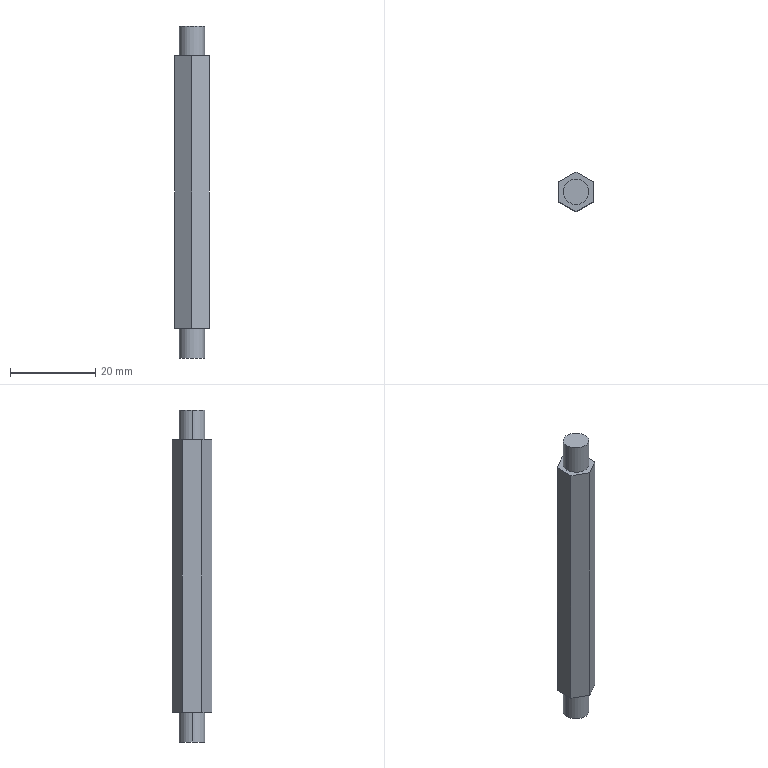Part | STEP file | 1 solid | 14 faces | box 8 x 9.238 x 78 mm | volume 3943 mm3 | plane 10 | cylinder 4 | commonest cylinder face diameters 6 x4
STEP:
#1=CARTESIAN_POINT('',(0.,0.,0.));
#2=DIRECTION('',(0.,0.,1.));
#3=DIRECTION('',(1.,0.,0.));
#4=AXIS2_PLACEMENT_3D('',#1,#2,#3);
#5=CARTESIAN_POINT('',(-5.42,-20.574,-50.535));
#6=VERTEX_POINT('',#5);
#7=CARTESIAN_POINT('',(-11.42,-20.574,-50.535));
#8=VERTEX_POINT('',#7);
#9=CARTESIAN_POINT('',(-8.42,-20.574,-50.535));
#10=DIRECTION('',(0.,0.,1.));
#11=DIRECTION('',(-1.,0.,0.));
#12=AXIS2_PLACEMENT_3D('',#9,#10,#11);
#13=CIRCLE('',#12,3.);
#14=CARTESIAN_POINT('',(-8.42,-20.574,-50.535));
#15=DIRECTION('',(0.,0.,-1.));
#16=DIRECTION('',(-1.,0.,0.));
#17=AXIS2_PLACEMENT_3D('',#14,#15,#16);
#18=CYLINDRICAL_SURFACE('',#17,3.);
#19=CARTESIAN_POINT('',(6.283,0.));
#20=DIRECTION('',(-1.,0.));
#21=VECTOR('',#20,1.);
#22=LINE('',#19,#21);
#23=(GEOMETRIC_REPRESENTATION_CONTEXT(2)PARAMETRIC_REPRESENTATION_CONTEXT()REPRESENTATION_CONTEXT('',''));
#24=DEFINITIONAL_REPRESENTATION('',(#22),#23);
#25=PCURVE('',#18,#24);
#26=CARTESIAN_POINT('',(-8.42,-20.574,-50.535));
#27=DIRECTION('',(0.,0.,-1.));
#28=DIRECTION('',(-1.,0.,0.));
#29=AXIS2_PLACEMENT_3D('',#26,#27,#28);
#30=PLANE('',#29);
#31=CARTESIAN_POINT('',(3.,0.));
#32=CARTESIAN_POINT('',(3.,-5.196));
#33=CARTESIAN_POINT('',(-1.5,-2.598));
#34=CARTESIAN_POINT('',(-6.,0.));
#35=CARTESIAN_POINT('',(-1.5,2.598));
#36=CARTESIAN_POINT('',(3.,5.196));
#37=CARTESIAN_POINT('',(3.,0.));
#38=(BOUNDED_CURVE()B_SPLINE_CURVE(2,(#31,#32,#33,#34,#35,#36,#37),.UNSPECIFIED.,.T.,.F.)B_SPLINE_CURVE_WITH_KNOTS((1,2,2,2,2,1),(-2.094,0.,2.094,4.189,6.283,8.378),.UNSPECIFIED.)CURVE()GEOMETRIC_REPRESENTATION_ITEM()RATIONAL_B_SPLINE_CURVE((1.,0.5,1.,0.5,1.,0.5,1.))REPRESENTATION_ITEM(''));
#39=(GEOMETRIC_REPRESENTATION_CONTEXT(2)PARAMETRIC_REPRESENTATION_CONTEXT()REPRESENTATION_CONTEXT('',''));
#40=DEFINITIONAL_REPRESENTATION('',(#38),#39);
#41=PCURVE('',#30,#40);
#42=SURFACE_CURVE('',#13,(#25,#41),.PCURVE_S1.);
#43=EDGE_CURVE('',#6,#8,#42,.T.);
#44=ORIENTED_EDGE('',*,*,#43,.F.);
#45=CARTESIAN_POINT('',(-5.42,-20.574,-57.535));
#46=VERTEX_POINT('',#45);
#47=CARTESIAN_POINT('',(-5.42,-20.574,-50.535));
#48=DIRECTION('',(0.,0.,-1.));
#49=VECTOR('',#48,1.);
#50=LINE('',#47,#49);
#51=CARTESIAN_POINT('',(3.142,0.));
#52=DIRECTION('',(0.,1.));
#53=VECTOR('',#52,1.);
#54=LINE('',#51,#53);
#55=(GEOMETRIC_REPRESENTATION_CONTEXT(2)PARAMETRIC_REPRESENTATION_CONTEXT()REPRESENTATION_CONTEXT('',''));
#56=DEFINITIONAL_REPRESENTATION('',(#54),#55);
#57=PCURVE('',#18,#56);
#58=CARTESIAN_POINT('',(-8.42,-20.574,-50.535));
#59=DIRECTION('',(0.,0.,-1.));
#60=DIRECTION('',(-1.,0.,0.));
#61=AXIS2_PLACEMENT_3D('',#58,#59,#60);
#62=CYLINDRICAL_SURFACE('',#61,3.);
#63=CARTESIAN_POINT('',(3.142,0.));
#64=DIRECTION('',(0.,1.));
#65=VECTOR('',#64,1.);
#66=LINE('',#63,#65);
#67=(GEOMETRIC_REPRESENTATION_CONTEXT(2)PARAMETRIC_REPRESENTATION_CONTEXT()REPRESENTATION_CONTEXT('',''));
#68=DEFINITIONAL_REPRESENTATION('',(#66),#67);
#69=PCURVE('',#62,#68);
#70=SURFACE_CURVE('',#50,(#57,#69),.PCURVE_S1.);
#71=EDGE_CURVE('',#6,#46,#70,.T.);
#72=ORIENTED_EDGE('',*,*,#71,.T.);
#73=CARTESIAN_POINT('',(-11.42,-20.574,-57.535));
#74=VERTEX_POINT('',#73);
#75=CARTESIAN_POINT('',(-8.42,-20.574,-57.535));
#76=DIRECTION('',(0.,0.,1.));
#77=DIRECTION('',(-1.,0.,0.));
#78=AXIS2_PLACEMENT_3D('',#75,#76,#77);
#79=CIRCLE('',#78,3.);
#80=CARTESIAN_POINT('',(6.283,7.));
#81=DIRECTION('',(-1.,0.));
#82=VECTOR('',#81,1.);
#83=LINE('',#80,#82);
#84=(GEOMETRIC_REPRESENTATION_CONTEXT(2)PARAMETRIC_REPRESENTATION_CONTEXT()REPRESENTATION_CONTEXT('',''));
#85=DEFINITIONAL_REPRESENTATION('',(#83),#84);
#86=PCURVE('',#18,#85);
#87=CARTESIAN_POINT('',(-8.42,-20.574,-57.535));
#88=DIRECTION('',(0.,0.,1.));
#89=DIRECTION('',(1.,0.,0.));
#90=AXIS2_PLACEMENT_3D('',#87,#88,#89);
#91=PLANE('',#90);
#92=CARTESIAN_POINT('',(0.,0.));
#93=DIRECTION('',(-1.,0.));
#94=AXIS2_PLACEMENT_2D('',#92,#93);
#95=CIRCLE('',#94,3.);
#96=(GEOMETRIC_REPRESENTATION_CONTEXT(2)PARAMETRIC_REPRESENTATION_CONTEXT()REPRESENTATION_CONTEXT('',''));
#97=DEFINITIONAL_REPRESENTATION('',(#95),#96);
#98=PCURVE('',#91,#97);
#99=SURFACE_CURVE('',#79,(#86,#98),.PCURVE_S1.);
#100=EDGE_CURVE('',#46,#74,#99,.T.);
#101=ORIENTED_EDGE('',*,*,#100,.T.);
#102=CARTESIAN_POINT('',(-11.42,-20.574,-50.535));
#103=DIRECTION('',(0.,0.,-1.));
#104=VECTOR('',#103,1.);
#105=LINE('',#102,#104);
#106=CARTESIAN_POINT('',(0.,0.));
#107=DIRECTION('',(0.,1.));
#108=VECTOR('',#107,1.);
#109=LINE('',#106,#108);
#110=(GEOMETRIC_REPRESENTATION_CONTEXT(2)PARAMETRIC_REPRESENTATION_CONTEXT()REPRESENTATION_CONTEXT('',''));
#111=DEFINITIONAL_REPRESENTATION('',(#109),#110);
#112=PCURVE('',#18,#111);
#113=CARTESIAN_POINT('',(6.283,0.));
#114=DIRECTION('',(0.,1.));
#115=VECTOR('',#114,1.);
#116=LINE('',#113,#115);
#117=(GEOMETRIC_REPRESENTATION_CONTEXT(2)PARAMETRIC_REPRESENTATION_CONTEXT()REPRESENTATION_CONTEXT('',''));
#118=DEFINITIONAL_REPRESENTATION('',(#116),#117);
#119=PCURVE('',#62,#118);
#120=SURFACE_CURVE('',#105,(#112,#119),.PCURVE_S1.);
#121=EDGE_CURVE('',#8,#74,#120,.T.);
#122=ORIENTED_EDGE('',*,*,#121,.F.);
#123=EDGE_LOOP('',(#44,#72,#101,#122));
#124=FACE_BOUND('',#123,.T.);
#125=ADVANCED_FACE('',(#124),#18,.T.);
#126=CARTESIAN_POINT('',(-11.42,-20.574,20.465));
#127=VERTEX_POINT('',#126);
#128=CARTESIAN_POINT('',(-5.42,-20.574,20.465));
#129=VERTEX_POINT('',#128);
#130=CARTESIAN_POINT('',(-8.42,-20.574,20.465));
#131=DIRECTION('',(0.,0.,-1.));
#132=DIRECTION('',(-1.,0.,0.));
#133=AXIS2_PLACEMENT_3D('',#130,#131,#132);
#134=CIRCLE('',#133,3.);
#135=CARTESIAN_POINT('',(-8.42,-20.574,13.465));
#136=DIRECTION('',(0.,0.,-1.));
#137=DIRECTION('',(-1.,0.,0.));
#138=AXIS2_PLACEMENT_3D('',#135,#136,#137);
#139=CYLINDRICAL_SURFACE('',#138,3.);
#140=CARTESIAN_POINT('',(0.,-7.));
#141=DIRECTION('',(1.,0.));
#142=VECTOR('',#141,1.);
#143=LINE('',#140,#142);
#144=(GEOMETRIC_REPRESENTATION_CONTEXT(2)PARAMETRIC_REPRESENTATION_CONTEXT()REPRESENTATION_CONTEXT('',''));
#145=DEFINITIONAL_REPRESENTATION('',(#143),#144);
#146=PCURVE('',#139,#145);
#147=CARTESIAN_POINT('',(-8.42,-20.574,20.465));
#148=DIRECTION('',(0.,0.,1.));
#149=DIRECTION('',(1.,0.,0.));
#150=AXIS2_PLACEMENT_3D('',#147,#148,#149);
#151=PLANE('',#150);
#152=CARTESIAN_POINT('',(-3.,0.));
#153=CARTESIAN_POINT('',(-3.,5.196));
#154=CARTESIAN_POINT('',(1.5,2.598));
#155=CARTESIAN_POINT('',(6.,0.));
#156=CARTESIAN_POINT('',(1.5,-2.598));
#157=CARTESIAN_POINT('',(-3.,-5.196));
#158=CARTESIAN_POINT('',(-3.,0.));
#159=(BOUNDED_CURVE()B_SPLINE_CURVE(2,(#152,#153,#154,#155,#156,#157,#158),.UNSPECIFIED.,.T.,.F.)B_SPLINE_CURVE_WITH_KNOTS((1,2,2,2,2,1),(-2.094,0.,2.094,4.189,6.283,8.378),.UNSPECIFIED.)CURVE()GEOMETRIC_REPRESENTATION_ITEM()RATIONAL_B_SPLINE_CURVE((1.,0.5,1.,0.5,1.,0.5,1.))REPRESENTATION_ITEM(''));
#160=(GEOMETRIC_REPRESENTATION_CONTEXT(2)PARAMETRIC_REPRESENTATION_CONTEXT()REPRESENTATION_CONTEXT('',''));
#161=DEFINITIONAL_REPRESENTATION('',(#159),#160);
#162=PCURVE('',#151,#161);
#163=SURFACE_CURVE('',#134,(#146,#162),.PCURVE_S1.);
#164=EDGE_CURVE('',#127,#129,#163,.T.);
#165=ORIENTED_EDGE('',*,*,#164,.T.);
#166=CARTESIAN_POINT('',(-5.42,-20.574,13.465));
#167=VERTEX_POINT('',#166);
#168=CARTESIAN_POINT('',(-5.42,-20.574,13.465));
#169=DIRECTION('',(0.,0.,-1.));
#170=VECTOR('',#169,1.);
#171=LINE('',#168,#170);
#172=CARTESIAN_POINT('',(3.142,0.));
#173=DIRECTION('',(0.,1.));
#174=VECTOR('',#173,1.);
#175=LINE('',#172,#174);
#176=(GEOMETRIC_REPRESENTATION_CONTEXT(2)PARAMETRIC_REPRESENTATION_CONTEXT()REPRESENTATION_CONTEXT('',''));
#177=DEFINITIONAL_REPRESENTATION('',(#175),#176);
#178=PCURVE('',#139,#177);
#179=CARTESIAN_POINT('',(-8.42,-20.574,13.465));
#180=DIRECTION('',(0.,0.,-1.));
#181=DIRECTION('',(-1.,0.,0.));
#182=AXIS2_PLACEMENT_3D('',#179,#180,#181);
#183=CYLINDRICAL_SURFACE('',#182,3.);
#184=CARTESIAN_POINT('',(3.142,0.));
#185=DIRECTION('',(0.,1.));
#186=VECTOR('',#185,1.);
#187=LINE('',#184,#186);
#188=(GEOMETRIC_REPRESENTATION_CONTEXT(2)PARAMETRIC_REPRESENTATION_CONTEXT()REPRESENTATION_CONTEXT('',''));
#189=DEFINITIONAL_REPRESENTATION('',(#187),#188);
#190=PCURVE('',#183,#189);
#191=SURFACE_CURVE('',#171,(#178,#190),.PCURVE_S1.);
#192=EDGE_CURVE('',#129,#167,#191,.T.);
#193=ORIENTED_EDGE('',*,*,#192,.T.);
#194=CARTESIAN_POINT('',(-11.42,-20.574,13.465));
#195=VERTEX_POINT('',#194);
#196=CARTESIAN_POINT('',(-8.42,-20.574,13.465));
#197=DIRECTION('',(0.,0.,-1.));
#198=DIRECTION('',(-1.,0.,0.));
#199=AXIS2_PLACEMENT_3D('',#196,#197,#198);
#200=CIRCLE('',#199,3.);
#201=CARTESIAN_POINT('',(0.,0.));
#202=DIRECTION('',(1.,0.));
#203=VECTOR('',#202,1.);
#204=LINE('',#201,#203);
#205=(GEOMETRIC_REPRESENTATION_CONTEXT(2)PARAMETRIC_REPRESENTATION_CONTEXT()REPRESENTATION_CONTEXT('',''));
#206=DEFINITIONAL_REPRESENTATION('',(#204),#205);
#207=PCURVE('',#139,#206);
#208=CARTESIAN_POINT('',(-8.42,-20.574,13.465));
#209=DIRECTION('',(0.,0.,1.));
#210=DIRECTION('',(1.,0.,0.));
#211=AXIS2_PLACEMENT_3D('',#208,#209,#210);
#212=PLANE('',#211);
#213=CARTESIAN_POINT('',(-3.,0.));
#214=CARTESIAN_POINT('',(-3.,5.196));
#215=CARTESIAN_POINT('',(1.5,2.598));
#216=CARTESIAN_POINT('',(6.,0.));
#217=CARTESIAN_POINT('',(1.5,-2.598));
#218=CARTESIAN_POINT('',(-3.,-5.196));
#219=CARTESIAN_POINT('',(-3.,0.));
#220=(BOUNDED_CURVE()B_SPLINE_CURVE(2,(#213,#214,#215,#216,#217,#218,#219),.UNSPECIFIED.,.T.,.F.)B_SPLINE_CURVE_WITH_KNOTS((1,2,2,2,2,1),(-2.094,0.,2.094,4.189,6.283,8.378),.UNSPECIFIED.)CURVE()GEOMETRIC_REPRESENTATION_ITEM()RATIONAL_B_SPLINE_CURVE((1.,0.5,1.,0.5,1.,0.5,1.))REPRESENTATION_ITEM(''));
#221=(GEOMETRIC_REPRESENTATION_CONTEXT(2)PARAMETRIC_REPRESENTATION_CONTEXT()REPRESENTATION_CONTEXT('',''));
#222=DEFINITIONAL_REPRESENTATION('',(#220),#221);
#223=PCURVE('',#212,#222);
#224=SURFACE_CURVE('',#200,(#207,#223),.PCURVE_S1.);
#225=EDGE_CURVE('',#195,#167,#224,.T.);
#226=ORIENTED_EDGE('',*,*,#225,.F.);
#227=CARTESIAN_POINT('',(-11.42,-20.574,13.465));
#228=DIRECTION('',(0.,0.,-1.));
#229=VECTOR('',#228,1.);
#230=LINE('',#227,#229);
#231=CARTESIAN_POINT('',(0.,0.));
#232=DIRECTION('',(0.,1.));
#233=VECTOR('',#232,1.);
#234=LINE('',#231,#233);
#235=(GEOMETRIC_REPRESENTATION_CONTEXT(2)PARAMETRIC_REPRESENTATION_CONTEXT()REPRESENTATION_CONTEXT('',''));
#236=DEFINITIONAL_REPRESENTATION('',(#234),#235);
#237=PCURVE('',#139,#236);
#238=CARTESIAN_POINT('',(6.283,0.));
#239=DIRECTION('',(0.,1.));
#240=VECTOR('',#239,1.);
#241=LINE('',#238,#240);
#242=(GEOMETRIC_REPRESENTATION_CONTEXT(2)PARAMETRIC_REPRESENTATION_CONTEXT()REPRESENTATION_CONTEXT('',''));
#243=DEFINITIONAL_REPRESENTATION('',(#241),#242);
#244=PCURVE('',#183,#243);
#245=SURFACE_CURVE('',#230,(#237,#244),.PCURVE_S1.);
#246=EDGE_CURVE('',#127,#195,#245,.T.);
#247=ORIENTED_EDGE('',*,*,#246,.F.);
#248=EDGE_LOOP('',(#165,#193,#226,#247));
#249=FACE_BOUND('',#248,.T.);
#250=ADVANCED_FACE('',(#249),#139,.T.);
#251=CARTESIAN_POINT('',(-8.42,-25.193,13.465));
#252=VERTEX_POINT('',#251);
#253=CARTESIAN_POINT('',(-8.42,-25.193,-50.535));
#254=VERTEX_POINT('',#253);
#255=CARTESIAN_POINT('',(-8.42,-25.193,-18.535));
#256=DIRECTION('',(0.,0.,-1.));
#257=VECTOR('',#256,1.);
#258=LINE('',#255,#257);
#259=CARTESIAN_POINT('',(-8.42,-25.193,-18.535));
#260=DIRECTION('',(0.5,-0.866,0.));
#261=DIRECTION('',(0.866,0.5,0.));
#262=AXIS2_PLACEMENT_3D('',#259,#260,#261);
#263=PLANE('',#262);
#264=CARTESIAN_POINT('',(0.,0.));
#265=DIRECTION('',(0.,-1.));
#266=VECTOR('',#265,1.);
#267=LINE('',#264,#266);
#268=(GEOMETRIC_REPRESENTATION_CONTEXT(2)PARAMETRIC_REPRESENTATION_CONTEXT()REPRESENTATION_CONTEXT('',''));
#269=DEFINITIONAL_REPRESENTATION('',(#267),#268);
#270=PCURVE('',#263,#269);
#271=CARTESIAN_POINT('',(-12.42,-22.883,-18.535));
#272=DIRECTION('',(-0.5,-0.866,0.));
#273=DIRECTION('',(0.866,-0.5,0.));
#274=AXIS2_PLACEMENT_3D('',#271,#272,#273);
#275=PLANE('',#274);
#276=CARTESIAN_POINT('',(4.619,0.));
#277=DIRECTION('',(0.,-1.));
#278=VECTOR('',#277,1.);
#279=LINE('',#276,#278);
#280=(GEOMETRIC_REPRESENTATION_CONTEXT(2)PARAMETRIC_REPRESENTATION_CONTEXT()REPRESENTATION_CONTEXT('',''));
#281=DEFINITIONAL_REPRESENTATION('',(#279),#280);
#282=PCURVE('',#275,#281);
#283=SURFACE_CURVE('',#258,(#270,#282),.PCURVE_S1.);
#284=EDGE_CURVE('',#252,#254,#283,.T.);
#285=ORIENTED_EDGE('',*,*,#284,.T.);
#286=CARTESIAN_POINT('',(-4.42,-22.883,-50.535));
#287=VERTEX_POINT('',#286);
#288=CARTESIAN_POINT('',(-8.42,-25.193,-50.535));
#289=DIRECTION('',(0.866,0.5,0.));
#290=VECTOR('',#289,1.);
#291=LINE('',#288,#290);
#292=CARTESIAN_POINT('',(0.,-32.));
#293=DIRECTION('',(1.,0.));
#294=VECTOR('',#293,1.);
#295=LINE('',#292,#294);
#296=(GEOMETRIC_REPRESENTATION_CONTEXT(2)PARAMETRIC_REPRESENTATION_CONTEXT()REPRESENTATION_CONTEXT('',''));
#297=DEFINITIONAL_REPRESENTATION('',(#295),#296);
#298=PCURVE('',#263,#297);
#299=CARTESIAN_POINT('',(0.,-4.619));
#300=DIRECTION('',(-0.866,0.5));
#301=VECTOR('',#300,1.);
#302=LINE('',#299,#301);
#303=(GEOMETRIC_REPRESENTATION_CONTEXT(2)PARAMETRIC_REPRESENTATION_CONTEXT()REPRESENTATION_CONTEXT('',''));
#304=DEFINITIONAL_REPRESENTATION('',(#302),#303);
#305=PCURVE('',#30,#304);
#306=SURFACE_CURVE('',#291,(#298,#305),.PCURVE_S1.);
#307=EDGE_CURVE('',#254,#287,#306,.T.);
#308=ORIENTED_EDGE('',*,*,#307,.T.);
#309=CARTESIAN_POINT('',(-4.42,-22.883,13.465));
#310=VERTEX_POINT('',#309);
#311=CARTESIAN_POINT('',(-4.42,-22.883,-18.535));
#312=DIRECTION('',(0.,0.,1.));
#313=VECTOR('',#312,1.);
#314=LINE('',#311,#313);
#315=CARTESIAN_POINT('',(4.619,0.));
#316=DIRECTION('',(0.,1.));
#317=VECTOR('',#316,1.);
#318=LINE('',#315,#317);
#319=(GEOMETRIC_REPRESENTATION_CONTEXT(2)PARAMETRIC_REPRESENTATION_CONTEXT()REPRESENTATION_CONTEXT('',''));
#320=DEFINITIONAL_REPRESENTATION('',(#318),#319);
#321=PCURVE('',#263,#320);
#322=CARTESIAN_POINT('',(-4.42,-22.883,-18.535));
#323=DIRECTION('',(1.,0.,0.));
#324=DIRECTION('',(0.,1.,0.));
#325=AXIS2_PLACEMENT_3D('',#322,#323,#324);
#326=PLANE('',#325);
#327=CARTESIAN_POINT('',(0.,0.));
#328=DIRECTION('',(0.,1.));
#329=VECTOR('',#328,1.);
#330=LINE('',#327,#329);
#331=(GEOMETRIC_REPRESENTATION_CONTEXT(2)PARAMETRIC_REPRESENTATION_CONTEXT()REPRESENTATION_CONTEXT('',''));
#332=DEFINITIONAL_REPRESENTATION('',(#330),#331);
#333=PCURVE('',#326,#332);
#334=SURFACE_CURVE('',#314,(#321,#333),.PCURVE_S1.);
#335=EDGE_CURVE('',#287,#310,#334,.T.);
#336=ORIENTED_EDGE('',*,*,#335,.T.);
#337=CARTESIAN_POINT('',(-8.42,-25.193,13.465));
#338=DIRECTION('',(-0.866,-0.5,0.));
#339=VECTOR('',#338,1.);
#340=LINE('',#337,#339);
#341=CARTESIAN_POINT('',(0.,32.));
#342=DIRECTION('',(-1.,0.));
#343=VECTOR('',#342,1.);
#344=LINE('',#341,#343);
#345=(GEOMETRIC_REPRESENTATION_CONTEXT(2)PARAMETRIC_REPRESENTATION_CONTEXT()REPRESENTATION_CONTEXT('',''));
#346=DEFINITIONAL_REPRESENTATION('',(#344),#345);
#347=PCURVE('',#263,#346);
#348=CARTESIAN_POINT('',(0.,-4.619));
#349=DIRECTION('',(-0.866,-0.5));
#350=VECTOR('',#349,1.);
#351=LINE('',#348,#350);
#352=(GEOMETRIC_REPRESENTATION_CONTEXT(2)PARAMETRIC_REPRESENTATION_CONTEXT()REPRESENTATION_CONTEXT('',''));
#353=DEFINITIONAL_REPRESENTATION('',(#351),#352);
#354=PCURVE('',#212,#353);
#355=SURFACE_CURVE('',#340,(#347,#354),.PCURVE_S1.);
#356=EDGE_CURVE('',#310,#252,#355,.T.);
#357=ORIENTED_EDGE('',*,*,#356,.T.);
#358=EDGE_LOOP('',(#285,#308,#336,#357));
#359=FACE_BOUND('',#358,.T.);
#360=ADVANCED_FACE('',(#359),#263,.T.);
#361=CARTESIAN_POINT('',(-12.42,-22.883,-50.535));
#362=VERTEX_POINT('',#361);
#363=CARTESIAN_POINT('',(-8.42,-25.193,-50.535));
#364=DIRECTION('',(-0.866,0.5,0.));
#365=VECTOR('',#364,1.);
#366=LINE('',#363,#365);
#367=CARTESIAN_POINT('',(0.,-4.619));
#368=DIRECTION('',(0.866,0.5));
#369=VECTOR('',#368,1.);
#370=LINE('',#367,#369);
#371=(GEOMETRIC_REPRESENTATION_CONTEXT(2)PARAMETRIC_REPRESENTATION_CONTEXT()REPRESENTATION_CONTEXT('',''));
#372=DEFINITIONAL_REPRESENTATION('',(#370),#371);
#373=PCURVE('',#30,#372);
#374=CARTESIAN_POINT('',(4.619,-32.));
#375=DIRECTION('',(-1.,0.));
#376=VECTOR('',#375,1.);
#377=LINE('',#374,#376);
#378=(GEOMETRIC_REPRESENTATION_CONTEXT(2)PARAMETRIC_REPRESENTATION_CONTEXT()REPRESENTATION_CONTEXT('',''));
#379=DEFINITIONAL_REPRESENTATION('',(#377),#378);
#380=PCURVE('',#275,#379);
#381=SURFACE_CURVE('',#366,(#373,#380),.PCURVE_S1.);
#382=EDGE_CURVE('',#254,#362,#381,.T.);
#383=ORIENTED_EDGE('',*,*,#382,.T.);
#384=CARTESIAN_POINT('',(-12.42,-18.264,-50.535));
#385=VERTEX_POINT('',#384);
#386=CARTESIAN_POINT('',(-12.42,-20.574,-50.535));
#387=DIRECTION('',(0.,1.,0.));
#388=VECTOR('',#387,1.);
#389=LINE('',#386,#388);
#390=CARTESIAN_POINT('',(4.,0.));
#391=DIRECTION('',(0.,1.));
#392=VECTOR('',#391,1.);
#393=LINE('',#390,#392);
#394=(GEOMETRIC_REPRESENTATION_CONTEXT(2)PARAMETRIC_REPRESENTATION_CONTEXT()REPRESENTATION_CONTEXT('',''));
#395=DEFINITIONAL_REPRESENTATION('',(#393),#394);
#396=PCURVE('',#30,#395);
#397=CARTESIAN_POINT('',(-12.42,-18.264,-18.535));
#398=DIRECTION('',(-1.,0.,0.));
#399=DIRECTION('',(0.,-1.,0.));
#400=AXIS2_PLACEMENT_3D('',#397,#398,#399);
#401=PLANE('',#400);
#402=CARTESIAN_POINT('',(2.309,-32.));
#403=DIRECTION('',(-1.,0.));
#404=VECTOR('',#403,1.);
#405=LINE('',#402,#404);
#406=(GEOMETRIC_REPRESENTATION_CONTEXT(2)PARAMETRIC_REPRESENTATION_CONTEXT()REPRESENTATION_CONTEXT('',''));
#407=DEFINITIONAL_REPRESENTATION('',(#405),#406);
#408=PCURVE('',#401,#407);
#409=SURFACE_CURVE('',#389,(#396,#408),.PCURVE_S1.);
#410=EDGE_CURVE('',#362,#385,#409,.T.);
#411=ORIENTED_EDGE('',*,*,#410,.T.);
#412=CARTESIAN_POINT('',(-8.42,-15.955,-50.535));
#413=VERTEX_POINT('',#412);
#414=CARTESIAN_POINT('',(-12.42,-18.264,-50.535));
#415=DIRECTION('',(0.866,0.5,0.));
#416=VECTOR('',#415,1.);
#417=LINE('',#414,#416);
#418=CARTESIAN_POINT('',(4.,2.309));
#419=DIRECTION('',(-0.866,0.5));
#420=VECTOR('',#419,1.);
#421=LINE('',#418,#420);
#422=(GEOMETRIC_REPRESENTATION_CONTEXT(2)PARAMETRIC_REPRESENTATION_CONTEXT()REPRESENTATION_CONTEXT('',''));
#423=DEFINITIONAL_REPRESENTATION('',(#421),#422);
#424=PCURVE('',#30,#423);
#425=CARTESIAN_POINT('',(-8.42,-15.955,-18.535));
#426=DIRECTION('',(-0.5,0.866,0.));
#427=DIRECTION('',(-0.866,-0.5,0.));
#428=AXIS2_PLACEMENT_3D('',#425,#426,#427);
#429=PLANE('',#428);
#430=CARTESIAN_POINT('',(4.619,-32.));
#431=DIRECTION('',(-1.,0.));
#432=VECTOR('',#431,1.);
#433=LINE('',#430,#432);
#434=(GEOMETRIC_REPRESENTATION_CONTEXT(2)PARAMETRIC_REPRESENTATION_CONTEXT()REPRESENTATION_CONTEXT('',''));
#435=DEFINITIONAL_REPRESENTATION('',(#433),#434);
#436=PCURVE('',#429,#435);
#437=SURFACE_CURVE('',#417,(#424,#436),.PCURVE_S1.);
#438=EDGE_CURVE('',#385,#413,#437,.T.);
#439=ORIENTED_EDGE('',*,*,#438,.T.);
#440=CARTESIAN_POINT('',(-4.42,-18.264,-50.535));
#441=VERTEX_POINT('',#440);
#442=CARTESIAN_POINT('',(-8.42,-15.955,-50.535));
#443=DIRECTION('',(0.866,-0.5,0.));
#444=VECTOR('',#443,1.);
#445=LINE('',#442,#444);
#446=CARTESIAN_POINT('',(0.,4.619));
#447=DIRECTION('',(-0.866,-0.5));
#448=VECTOR('',#447,1.);
#449=LINE('',#446,#448);
#450=(GEOMETRIC_REPRESENTATION_CONTEXT(2)PARAMETRIC_REPRESENTATION_CONTEXT()REPRESENTATION_CONTEXT('',''));
#451=DEFINITIONAL_REPRESENTATION('',(#449),#450);
#452=PCURVE('',#30,#451);
#453=CARTESIAN_POINT('',(-4.42,-18.264,-18.535));
#454=DIRECTION('',(0.5,0.866,0.));
#455=DIRECTION('',(-0.866,0.5,0.));
#456=AXIS2_PLACEMENT_3D('',#453,#454,#455);
#457=PLANE('',#456);
#458=CARTESIAN_POINT('',(4.619,-32.));
#459=DIRECTION('',(-1.,0.));
#460=VECTOR('',#459,1.);
#461=LINE('',#458,#460);
#462=(GEOMETRIC_REPRESENTATION_CONTEXT(2)PARAMETRIC_REPRESENTATION_CONTEXT()REPRESENTATION_CONTEXT('',''));
#463=DEFINITIONAL_REPRESENTATION('',(#461),#462);
#464=PCURVE('',#457,#463);
#465=SURFACE_CURVE('',#445,(#452,#464),.PCURVE_S1.);
#466=EDGE_CURVE('',#413,#441,#465,.T.);
#467=ORIENTED_EDGE('',*,*,#466,.T.);
#468=CARTESIAN_POINT('',(-4.42,-20.574,-50.535));
#469=DIRECTION('',(0.,-1.,0.));
#470=VECTOR('',#469,1.);
#471=LINE('',#468,#470);
#472=CARTESIAN_POINT('',(-4.,0.));
#473=DIRECTION('',(0.,-1.));
#474=VECTOR('',#473,1.);
#475=LINE('',#472,#474);
#476=(GEOMETRIC_REPRESENTATION_CONTEXT(2)PARAMETRIC_REPRESENTATION_CONTEXT()REPRESENTATION_CONTEXT('',''));
#477=DEFINITIONAL_REPRESENTATION('',(#475),#476);
#478=PCURVE('',#30,#477);
#479=CARTESIAN_POINT('',(2.309,-32.));
#480=DIRECTION('',(-1.,0.));
#481=VECTOR('',#480,1.);
#482=LINE('',#479,#481);
#483=(GEOMETRIC_REPRESENTATION_CONTEXT(2)PARAMETRIC_REPRESENTATION_CONTEXT()REPRESENTATION_CONTEXT('',''));
#484=DEFINITIONAL_REPRESENTATION('',(#482),#483);
#485=PCURVE('',#326,#484);
#486=SURFACE_CURVE('',#471,(#478,#485),.PCURVE_S1.);
#487=EDGE_CURVE('',#441,#287,#486,.T.);
#488=ORIENTED_EDGE('',*,*,#487,.T.);
#489=ORIENTED_EDGE('',*,*,#307,.F.);
#490=EDGE_LOOP('',(#383,#411,#439,#467,#488,#489));
#491=FACE_BOUND('',#490,.T.);
#492=CARTESIAN_POINT('',(-8.42,-20.574,-50.535));
#493=DIRECTION('',(0.,0.,1.));
#494=DIRECTION('',(-1.,0.,0.));
#495=AXIS2_PLACEMENT_3D('',#492,#493,#494);
#496=CIRCLE('',#495,3.);
#497=CARTESIAN_POINT('',(3.,0.));
#498=CARTESIAN_POINT('',(3.,-5.196));
#499=CARTESIAN_POINT('',(-1.5,-2.598));
#500=CARTESIAN_POINT('',(-6.,0.));
#501=CARTESIAN_POINT('',(-1.5,2.598));
#502=CARTESIAN_POINT('',(3.,5.196));
#503=CARTESIAN_POINT('',(3.,0.));
#504=(BOUNDED_CURVE()B_SPLINE_CURVE(2,(#497,#498,#499,#500,#501,#502,#503),.UNSPECIFIED.,.T.,.F.)B_SPLINE_CURVE_WITH_KNOTS((1,2,2,2,2,1),(-2.094,0.,2.094,4.189,6.283,8.378),.UNSPECIFIED.)CURVE()GEOMETRIC_REPRESENTATION_ITEM()RATIONAL_B_SPLINE_CURVE((1.,0.5,1.,0.5,1.,0.5,1.))REPRESENTATION_ITEM(''));
#505=(GEOMETRIC_REPRESENTATION_CONTEXT(2)PARAMETRIC_REPRESENTATION_CONTEXT()REPRESENTATION_CONTEXT('',''));
#506=DEFINITIONAL_REPRESENTATION('',(#504),#505);
#507=PCURVE('',#30,#506);
#508=CARTESIAN_POINT('',(6.283,0.));
#509=DIRECTION('',(-1.,0.));
#510=VECTOR('',#509,1.);
#511=LINE('',#508,#510);
#512=(GEOMETRIC_REPRESENTATION_CONTEXT(2)PARAMETRIC_REPRESENTATION_CONTEXT()REPRESENTATION_CONTEXT('',''));
#513=DEFINITIONAL_REPRESENTATION('',(#511),#512);
#514=PCURVE('',#62,#513);
#515=SURFACE_CURVE('',#496,(#507,#514),.PCURVE_S1.);
#516=EDGE_CURVE('',#8,#6,#515,.T.);
#517=ORIENTED_EDGE('',*,*,#516,.T.);
#518=ORIENTED_EDGE('',*,*,#43,.T.);
#519=EDGE_LOOP('',(#517,#518));
#520=FACE_BOUND('',#519,.T.);
#521=ADVANCED_FACE('',(#491,#520),#30,.T.);
#522=CARTESIAN_POINT('',(-12.42,-22.883,13.465));
#523=VERTEX_POINT('',#522);
#524=CARTESIAN_POINT('',(-12.42,-22.883,-18.535));
#525=DIRECTION('',(0.,0.,-1.));
#526=VECTOR('',#525,1.);
#527=LINE('',#524,#526);
#528=CARTESIAN_POINT('',(0.,0.));
#529=DIRECTION('',(0.,-1.));
#530=VECTOR('',#529,1.);
#531=LINE('',#528,#530);
#532=(GEOMETRIC_REPRESENTATION_CONTEXT(2)PARAMETRIC_REPRESENTATION_CONTEXT()REPRESENTATION_CONTEXT('',''));
#533=DEFINITIONAL_REPRESENTATION('',(#531),#532);
#534=PCURVE('',#275,#533);
#535=CARTESIAN_POINT('',(4.619,0.));
#536=DIRECTION('',(0.,-1.));
#537=VECTOR('',#536,1.);
#538=LINE('',#535,#537);
#539=(GEOMETRIC_REPRESENTATION_CONTEXT(2)PARAMETRIC_REPRESENTATION_CONTEXT()REPRESENTATION_CONTEXT('',''));
#540=DEFINITIONAL_REPRESENTATION('',(#538),#539);
#541=PCURVE('',#401,#540);
#542=SURFACE_CURVE('',#527,(#534,#541),.PCURVE_S1.);
#543=EDGE_CURVE('',#523,#362,#542,.T.);
#544=ORIENTED_EDGE('',*,*,#543,.T.);
#545=ORIENTED_EDGE('',*,*,#382,.F.);
#546=ORIENTED_EDGE('',*,*,#284,.F.);
#547=CARTESIAN_POINT('',(-12.42,-22.883,13.465));
#548=DIRECTION('',(-0.866,0.5,0.));
#549=VECTOR('',#548,1.);
#550=LINE('',#547,#549);
#551=CARTESIAN_POINT('',(0.,32.));
#552=DIRECTION('',(-1.,0.));
#553=VECTOR('',#552,1.);
#554=LINE('',#551,#553);
#555=(GEOMETRIC_REPRESENTATION_CONTEXT(2)PARAMETRIC_REPRESENTATION_CONTEXT()REPRESENTATION_CONTEXT('',''));
#556=DEFINITIONAL_REPRESENTATION('',(#554),#555);
#557=PCURVE('',#275,#556);
#558=CARTESIAN_POINT('',(-4.,-2.309));
#559=DIRECTION('',(-0.866,0.5));
#560=VECTOR('',#559,1.);
#561=LINE('',#558,#560);
#562=(GEOMETRIC_REPRESENTATION_CONTEXT(2)PARAMETRIC_REPRESENTATION_CONTEXT()REPRESENTATION_CONTEXT('',''));
#563=DEFINITIONAL_REPRESENTATION('',(#561),#562);
#564=PCURVE('',#212,#563);
#565=SURFACE_CURVE('',#550,(#557,#564),.PCURVE_S1.);
#566=EDGE_CURVE('',#252,#523,#565,.T.);
#567=ORIENTED_EDGE('',*,*,#566,.T.);
#568=EDGE_LOOP('',(#544,#545,#546,#567));
#569=FACE_BOUND('',#568,.T.);
#570=ADVANCED_FACE('',(#569),#275,.T.);
#571=CARTESIAN_POINT('',(-4.42,-18.264,13.465));
#572=VERTEX_POINT('',#571);
#573=CARTESIAN_POINT('',(-4.42,-20.574,13.465));
#574=DIRECTION('',(0.,1.,0.));
#575=VECTOR('',#574,1.);
#576=LINE('',#573,#575);
#577=CARTESIAN_POINT('',(4.,0.));
#578=DIRECTION('',(0.,1.));
#579=VECTOR('',#578,1.);
#580=LINE('',#577,#579);
#581=(GEOMETRIC_REPRESENTATION_CONTEXT(2)PARAMETRIC_REPRESENTATION_CONTEXT()REPRESENTATION_CONTEXT('',''));
#582=DEFINITIONAL_REPRESENTATION('',(#580),#581);
#583=PCURVE('',#212,#582);
#584=CARTESIAN_POINT('',(2.309,32.));
#585=DIRECTION('',(1.,0.));
#586=VECTOR('',#585,1.);
#587=LINE('',#584,#586);
#588=(GEOMETRIC_REPRESENTATION_CONTEXT(2)PARAMETRIC_REPRESENTATION_CONTEXT()REPRESENTATION_CONTEXT('',''));
#589=DEFINITIONAL_REPRESENTATION('',(#587),#588);
#590=PCURVE('',#326,#589);
#591=SURFACE_CURVE('',#576,(#583,#590),.PCURVE_S1.);
#592=EDGE_CURVE('',#310,#572,#591,.T.);
#593=ORIENTED_EDGE('',*,*,#592,.T.);
#594=CARTESIAN_POINT('',(-8.42,-15.955,13.465));
#595=VERTEX_POINT('',#594);
#596=CARTESIAN_POINT('',(-4.42,-18.264,13.465));
#597=DIRECTION('',(-0.866,0.5,0.));
#598=VECTOR('',#597,1.);
#599=LINE('',#596,#598);
#600=CARTESIAN_POINT('',(4.,2.309));
#601=DIRECTION('',(-0.866,0.5));
#602=VECTOR('',#601,1.);
#603=LINE('',#600,#602);
#604=(GEOMETRIC_REPRESENTATION_CONTEXT(2)PARAMETRIC_REPRESENTATION_CONTEXT()REPRESENTATION_CONTEXT('',''));
#605=DEFINITIONAL_REPRESENTATION('',(#603),#604);
#606=PCURVE('',#212,#605);
#607=CARTESIAN_POINT('',(0.,32.));
#608=DIRECTION('',(1.,0.));
#609=VECTOR('',#608,1.);
#610=LINE('',#607,#609);
#611=(GEOMETRIC_REPRESENTATION_CONTEXT(2)PARAMETRIC_REPRESENTATION_CONTEXT()REPRESENTATION_CONTEXT('',''));
#612=DEFINITIONAL_REPRESENTATION('',(#610),#611);
#613=PCURVE('',#457,#612);
#614=SURFACE_CURVE('',#599,(#606,#613),.PCURVE_S1.);
#615=EDGE_CURVE('',#572,#595,#614,.T.);
#616=ORIENTED_EDGE('',*,*,#615,.T.);
#617=CARTESIAN_POINT('',(-12.42,-18.264,13.465));
#618=VERTEX_POINT('',#617);
#619=CARTESIAN_POINT('',(-8.42,-15.955,13.465));
#620=DIRECTION('',(-0.866,-0.5,0.));
#621=VECTOR('',#620,1.);
#622=LINE('',#619,#621);
#623=CARTESIAN_POINT('',(0.,4.619));
#624=DIRECTION('',(-0.866,-0.5));
#625=VECTOR('',#624,1.);
#626=LINE('',#623,#625);
#627=(GEOMETRIC_REPRESENTATION_CONTEXT(2)PARAMETRIC_REPRESENTATION_CONTEXT()REPRESENTATION_CONTEXT('',''));
#628=DEFINITIONAL_REPRESENTATION('',(#626),#627);
#629=PCURVE('',#212,#628);
#630=CARTESIAN_POINT('',(0.,32.));
#631=DIRECTION('',(1.,0.));
#632=VECTOR('',#631,1.);
#633=LINE('',#630,#632);
#634=(GEOMETRIC_REPRESENTATION_CONTEXT(2)PARAMETRIC_REPRESENTATION_CONTEXT()REPRESENTATION_CONTEXT('',''));
#635=DEFINITIONAL_REPRESENTATION('',(#633),#634);
#636=PCURVE('',#429,#635);
#637=SURFACE_CURVE('',#622,(#629,#636),.PCURVE_S1.);
#638=EDGE_CURVE('',#595,#618,#637,.T.);
#639=ORIENTED_EDGE('',*,*,#638,.T.);
#640=CARTESIAN_POINT('',(-12.42,-20.574,13.465));
#641=DIRECTION('',(0.,-1.,0.));
#642=VECTOR('',#641,1.);
#643=LINE('',#640,#642);
#644=CARTESIAN_POINT('',(-4.,0.));
#645=DIRECTION('',(0.,-1.));
#646=VECTOR('',#645,1.);
#647=LINE('',#644,#646);
#648=(GEOMETRIC_REPRESENTATION_CONTEXT(2)PARAMETRIC_REPRESENTATION_CONTEXT()REPRESENTATION_CONTEXT('',''));
#649=DEFINITIONAL_REPRESENTATION('',(#647),#648);
#650=PCURVE('',#212,#649);
#651=CARTESIAN_POINT('',(2.309,32.));
#652=DIRECTION('',(1.,0.));
#653=VECTOR('',#652,1.);
#654=LINE('',#651,#653);
#655=(GEOMETRIC_REPRESENTATION_CONTEXT(2)PARAMETRIC_REPRESENTATION_CONTEXT()REPRESENTATION_CONTEXT('',''));
#656=DEFINITIONAL_REPRESENTATION('',(#654),#655);
#657=PCURVE('',#401,#656);
#658=SURFACE_CURVE('',#643,(#650,#657),.PCURVE_S1.);
#659=EDGE_CURVE('',#618,#523,#658,.T.);
#660=ORIENTED_EDGE('',*,*,#659,.T.);
#661=ORIENTED_EDGE('',*,*,#566,.F.);
#662=ORIENTED_EDGE('',*,*,#356,.F.);
#663=EDGE_LOOP('',(#593,#616,#639,#660,#661,#662));
#664=FACE_BOUND('',#663,.T.);
#665=ORIENTED_EDGE('',*,*,#225,.T.);
#666=CARTESIAN_POINT('',(-8.42,-20.574,13.465));
#667=DIRECTION('',(0.,0.,-1.));
#668=DIRECTION('',(-1.,0.,0.));
#669=AXIS2_PLACEMENT_3D('',#666,#667,#668);
#670=CIRCLE('',#669,3.);
#671=CARTESIAN_POINT('',(-3.,0.));
#672=CARTESIAN_POINT('',(-3.,5.196));
#673=CARTESIAN_POINT('',(1.5,2.598));
#674=CARTESIAN_POINT('',(6.,0.));
#675=CARTESIAN_POINT('',(1.5,-2.598));
#676=CARTESIAN_POINT('',(-3.,-5.196));
#677=CARTESIAN_POINT('',(-3.,0.));
#678=(BOUNDED_CURVE()B_SPLINE_CURVE(2,(#671,#672,#673,#674,#675,#676,#677),.UNSPECIFIED.,.T.,.F.)B_SPLINE_CURVE_WITH_KNOTS((1,2,2,2,2,1),(-2.094,0.,2.094,4.189,6.283,8.378),.UNSPECIFIED.)CURVE()GEOMETRIC_REPRESENTATION_ITEM()RATIONAL_B_SPLINE_CURVE((1.,0.5,1.,0.5,1.,0.5,1.))REPRESENTATION_ITEM(''));
#679=(GEOMETRIC_REPRESENTATION_CONTEXT(2)PARAMETRIC_REPRESENTATION_CONTEXT()REPRESENTATION_CONTEXT('',''));
#680=DEFINITIONAL_REPRESENTATION('',(#678),#679);
#681=PCURVE('',#212,#680);
#682=CARTESIAN_POINT('',(0.,0.));
#683=DIRECTION('',(1.,0.));
#684=VECTOR('',#683,1.);
#685=LINE('',#682,#684);
#686=(GEOMETRIC_REPRESENTATION_CONTEXT(2)PARAMETRIC_REPRESENTATION_CONTEXT()REPRESENTATION_CONTEXT('',''));
#687=DEFINITIONAL_REPRESENTATION('',(#685),#686);
#688=PCURVE('',#183,#687);
#689=SURFACE_CURVE('',#670,(#681,#688),.PCURVE_S1.);
#690=EDGE_CURVE('',#167,#195,#689,.T.);
#691=ORIENTED_EDGE('',*,*,#690,.T.);
#692=EDGE_LOOP('',(#665,#691));
#693=FACE_BOUND('',#692,.T.);
#694=ADVANCED_FACE('',(#664,#693),#212,.T.);
#695=ORIENTED_EDGE('',*,*,#335,.F.);
#696=ORIENTED_EDGE('',*,*,#487,.F.);
#697=CARTESIAN_POINT('',(-4.42,-18.264,-18.535));
#698=DIRECTION('',(0.,0.,1.));
#699=VECTOR('',#698,1.);
#700=LINE('',#697,#699);
#701=CARTESIAN_POINT('',(4.619,0.));
#702=DIRECTION('',(0.,1.));
#703=VECTOR('',#702,1.);
#704=LINE('',#701,#703);
#705=(GEOMETRIC_REPRESENTATION_CONTEXT(2)PARAMETRIC_REPRESENTATION_CONTEXT()REPRESENTATION_CONTEXT('',''));
#706=DEFINITIONAL_REPRESENTATION('',(#704),#705);
#707=PCURVE('',#326,#706);
#708=CARTESIAN_POINT('',(0.,0.));
#709=DIRECTION('',(0.,1.));
#710=VECTOR('',#709,1.);
#711=LINE('',#708,#710);
#712=(GEOMETRIC_REPRESENTATION_CONTEXT(2)PARAMETRIC_REPRESENTATION_CONTEXT()REPRESENTATION_CONTEXT('',''));
#713=DEFINITIONAL_REPRESENTATION('',(#711),#712);
#714=PCURVE('',#457,#713);
#715=SURFACE_CURVE('',#700,(#707,#714),.PCURVE_S1.);
#716=EDGE_CURVE('',#441,#572,#715,.T.);
#717=ORIENTED_EDGE('',*,*,#716,.T.);
#718=ORIENTED_EDGE('',*,*,#592,.F.);
#719=EDGE_LOOP('',(#695,#696,#717,#718));
#720=FACE_BOUND('',#719,.T.);
#721=ADVANCED_FACE('',(#720),#326,.T.);
#722=CARTESIAN_POINT('',(-12.42,-18.264,-18.535));
#723=DIRECTION('',(0.,0.,-1.));
#724=VECTOR('',#723,1.);
#725=LINE('',#722,#724);
#726=CARTESIAN_POINT('',(0.,0.));
#727=DIRECTION('',(0.,-1.));
#728=VECTOR('',#727,1.);
#729=LINE('',#726,#728);
#730=(GEOMETRIC_REPRESENTATION_CONTEXT(2)PARAMETRIC_REPRESENTATION_CONTEXT()REPRESENTATION_CONTEXT('',''));
#731=DEFINITIONAL_REPRESENTATION('',(#729),#730);
#732=PCURVE('',#401,#731);
#733=CARTESIAN_POINT('',(4.619,0.));
#734=DIRECTION('',(0.,-1.));
#735=VECTOR('',#734,1.);
#736=LINE('',#733,#735);
#737=(GEOMETRIC_REPRESENTATION_CONTEXT(2)PARAMETRIC_REPRESENTATION_CONTEXT()REPRESENTATION_CONTEXT('',''));
#738=DEFINITIONAL_REPRESENTATION('',(#736),#737);
#739=PCURVE('',#429,#738);
#740=SURFACE_CURVE('',#725,(#732,#739),.PCURVE_S1.);
#741=EDGE_CURVE('',#618,#385,#740,.T.);
#742=ORIENTED_EDGE('',*,*,#741,.T.);
#743=ORIENTED_EDGE('',*,*,#410,.F.);
#744=ORIENTED_EDGE('',*,*,#543,.F.);
#745=ORIENTED_EDGE('',*,*,#659,.F.);
#746=EDGE_LOOP('',(#742,#743,#744,#745));
#747=FACE_BOUND('',#746,.T.);
#748=ADVANCED_FACE('',(#747),#401,.T.);
#749=ORIENTED_EDGE('',*,*,#716,.F.);
#750=ORIENTED_EDGE('',*,*,#466,.F.);
#751=CARTESIAN_POINT('',(-8.42,-15.955,-18.535));
#752=DIRECTION('',(0.,0.,1.));
#753=VECTOR('',#752,1.);
#754=LINE('',#751,#753);
#755=CARTESIAN_POINT('',(4.619,0.));
#756=DIRECTION('',(0.,1.));
#757=VECTOR('',#756,1.);
#758=LINE('',#755,#757);
#759=(GEOMETRIC_REPRESENTATION_CONTEXT(2)PARAMETRIC_REPRESENTATION_CONTEXT()REPRESENTATION_CONTEXT('',''));
#760=DEFINITIONAL_REPRESENTATION('',(#758),#759);
#761=PCURVE('',#457,#760);
#762=CARTESIAN_POINT('',(0.,0.));
#763=DIRECTION('',(0.,1.));
#764=VECTOR('',#763,1.);
#765=LINE('',#762,#764);
#766=(GEOMETRIC_REPRESENTATION_CONTEXT(2)PARAMETRIC_REPRESENTATION_CONTEXT()REPRESENTATION_CONTEXT('',''));
#767=DEFINITIONAL_REPRESENTATION('',(#765),#766);
#768=PCURVE('',#429,#767);
#769=SURFACE_CURVE('',#754,(#761,#768),.PCURVE_S1.);
#770=EDGE_CURVE('',#413,#595,#769,.T.);
#771=ORIENTED_EDGE('',*,*,#770,.T.);
#772=ORIENTED_EDGE('',*,*,#615,.F.);
#773=EDGE_LOOP('',(#749,#750,#771,#772));
#774=FACE_BOUND('',#773,.T.);
#775=ADVANCED_FACE('',(#774),#457,.T.);
#776=ORIENTED_EDGE('',*,*,#770,.F.);
#777=ORIENTED_EDGE('',*,*,#438,.F.);
#778=ORIENTED_EDGE('',*,*,#741,.F.);
#779=ORIENTED_EDGE('',*,*,#638,.F.);
#780=EDGE_LOOP('',(#776,#777,#778,#779));
#781=FACE_BOUND('',#780,.T.);
#782=ADVANCED_FACE('',(#781),#429,.T.);
#783=ORIENTED_EDGE('',*,*,#71,.F.);
#784=ORIENTED_EDGE('',*,*,#516,.F.);
#785=ORIENTED_EDGE('',*,*,#121,.T.);
#786=CARTESIAN_POINT('',(-8.42,-20.574,-57.535));
#787=DIRECTION('',(0.,0.,1.));
#788=DIRECTION('',(-1.,0.,0.));
#789=AXIS2_PLACEMENT_3D('',#786,#787,#788);
#790=CIRCLE('',#789,3.);
#791=CARTESIAN_POINT('',(6.283,7.));
#792=DIRECTION('',(-1.,0.));
#793=VECTOR('',#792,1.);
#794=LINE('',#791,#793);
#795=(GEOMETRIC_REPRESENTATION_CONTEXT(2)PARAMETRIC_REPRESENTATION_CONTEXT()REPRESENTATION_CONTEXT('',''));
#796=DEFINITIONAL_REPRESENTATION('',(#794),#795);
#797=PCURVE('',#62,#796);
#798=CARTESIAN_POINT('',(0.,0.));
#799=DIRECTION('',(-1.,0.));
#800=AXIS2_PLACEMENT_2D('',#798,#799);
#801=CIRCLE('',#800,3.);
#802=(GEOMETRIC_REPRESENTATION_CONTEXT(2)PARAMETRIC_REPRESENTATION_CONTEXT()REPRESENTATION_CONTEXT('',''));
#803=DEFINITIONAL_REPRESENTATION('',(#801),#802);
#804=PCURVE('',#91,#803);
#805=SURFACE_CURVE('',#790,(#797,#804),.PCURVE_S1.);
#806=EDGE_CURVE('',#74,#46,#805,.T.);
#807=ORIENTED_EDGE('',*,*,#806,.T.);
#808=EDGE_LOOP('',(#783,#784,#785,#807));
#809=FACE_BOUND('',#808,.T.);
#810=ADVANCED_FACE('',(#809),#62,.T.);
#811=ORIENTED_EDGE('',*,*,#192,.F.);
#812=CARTESIAN_POINT('',(-8.42,-20.574,20.465));
#813=DIRECTION('',(0.,0.,-1.));
#814=DIRECTION('',(-1.,0.,0.));
#815=AXIS2_PLACEMENT_3D('',#812,#813,#814);
#816=CIRCLE('',#815,3.);
#817=CARTESIAN_POINT('',(0.,-7.));
#818=DIRECTION('',(1.,0.));
#819=VECTOR('',#818,1.);
#820=LINE('',#817,#819);
#821=(GEOMETRIC_REPRESENTATION_CONTEXT(2)PARAMETRIC_REPRESENTATION_CONTEXT()REPRESENTATION_CONTEXT('',''));
#822=DEFINITIONAL_REPRESENTATION('',(#820),#821);
#823=PCURVE('',#183,#822);
#824=CARTESIAN_POINT('',(-3.,0.));
#825=CARTESIAN_POINT('',(-3.,5.196));
#826=CARTESIAN_POINT('',(1.5,2.598));
#827=CARTESIAN_POINT('',(6.,0.));
#828=CARTESIAN_POINT('',(1.5,-2.598));
#829=CARTESIAN_POINT('',(-3.,-5.196));
#830=CARTESIAN_POINT('',(-3.,0.));
#831=(BOUNDED_CURVE()B_SPLINE_CURVE(2,(#824,#825,#826,#827,#828,#829,#830),.UNSPECIFIED.,.T.,.F.)B_SPLINE_CURVE_WITH_KNOTS((1,2,2,2,2,1),(-2.094,0.,2.094,4.189,6.283,8.378),.UNSPECIFIED.)CURVE()GEOMETRIC_REPRESENTATION_ITEM()RATIONAL_B_SPLINE_CURVE((1.,0.5,1.,0.5,1.,0.5,1.))REPRESENTATION_ITEM(''));
#832=(GEOMETRIC_REPRESENTATION_CONTEXT(2)PARAMETRIC_REPRESENTATION_CONTEXT()REPRESENTATION_CONTEXT('',''));
#833=DEFINITIONAL_REPRESENTATION('',(#831),#832);
#834=PCURVE('',#151,#833);
#835=SURFACE_CURVE('',#816,(#823,#834),.PCURVE_S1.);
#836=EDGE_CURVE('',#129,#127,#835,.T.);
#837=ORIENTED_EDGE('',*,*,#836,.T.);
#838=ORIENTED_EDGE('',*,*,#246,.T.);
#839=ORIENTED_EDGE('',*,*,#690,.F.);
#840=EDGE_LOOP('',(#811,#837,#838,#839));
#841=FACE_BOUND('',#840,.T.);
#842=ADVANCED_FACE('',(#841),#183,.T.);
#843=ORIENTED_EDGE('',*,*,#806,.F.);
#844=ORIENTED_EDGE('',*,*,#100,.F.);
#845=EDGE_LOOP('',(#843,#844));
#846=FACE_BOUND('',#845,.T.);
#847=ADVANCED_FACE('',(#846),#91,.F.);
#848=ORIENTED_EDGE('',*,*,#164,.F.);
#849=ORIENTED_EDGE('',*,*,#836,.F.);
#850=EDGE_LOOP('',(#848,#849));
#851=FACE_BOUND('',#850,.T.);
#852=ADVANCED_FACE('',(#851),#151,.T.);
#853=CLOSED_SHELL('',(#125,#250,#360,#521,#570,#694,#721,#748,#775,#782,#810,#842,#847,#852));
#854=MANIFOLD_SOLID_BREP('',#853);
#855=(LENGTH_UNIT()NAMED_UNIT(*)SI_UNIT(.MILLI.,.METRE.));
#856=UNCERTAINTY_MEASURE_WITH_UNIT(LENGTH_MEASURE(0.0000001),#855,'','');
#857=(NAMED_UNIT(*)PLANE_ANGLE_UNIT()SI_UNIT($,.RADIAN.));
#858=(NAMED_UNIT(*)SI_UNIT($,.STERADIAN.)SOLID_ANGLE_UNIT());
#859=(GEOMETRIC_REPRESENTATION_CONTEXT(3)GLOBAL_UNCERTAINTY_ASSIGNED_CONTEXT((#856))GLOBAL_UNIT_ASSIGNED_CONTEXT((#855,#857,#858))REPRESENTATION_CONTEXT('',''));
#860=ADVANCED_BREP_SHAPE_REPRESENTATION('',(#4,#854),#859);